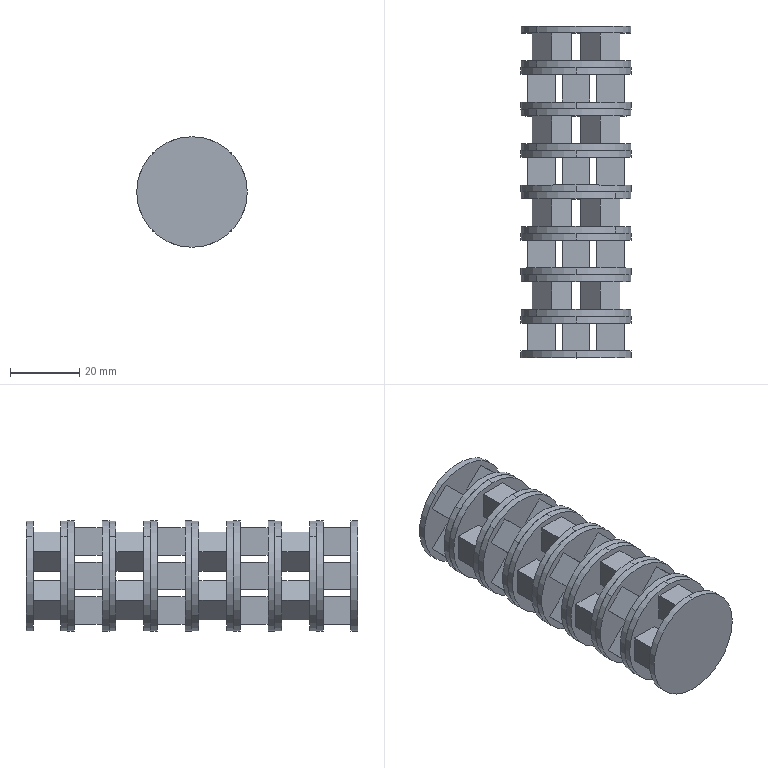Part | SolidWorks | 8 solids | 192 faces | box 32 x 96 x 32 mm | volume 42120 mm3 | plane 160 | cylinder 32 | commonest cylinder face diameters 32 x32